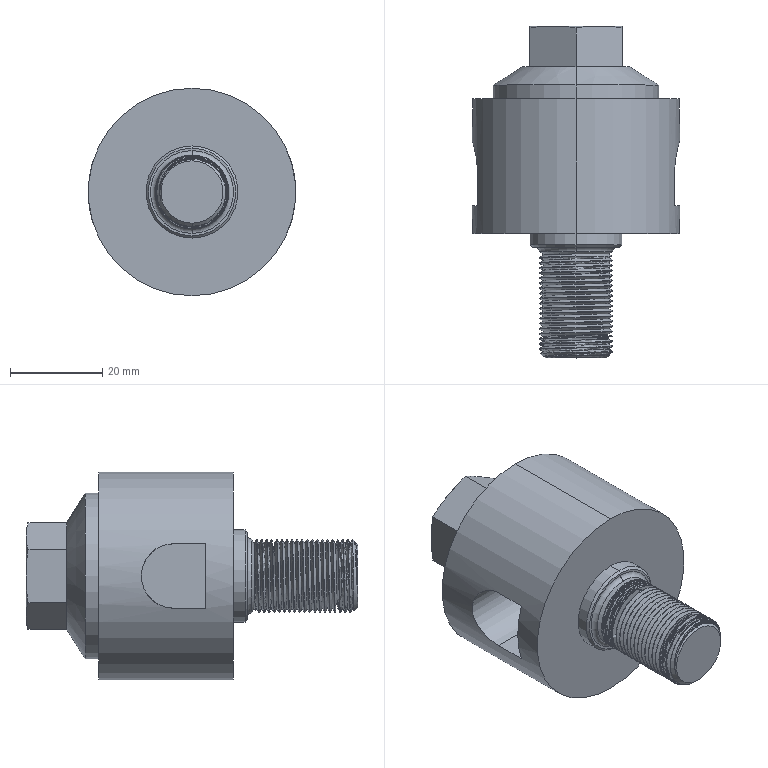Part | STEP file | Parafuso DSR-C - M16 | 1 solid | 96 faces | box 45 x 72 x 45 mm | volume 55144 mm3 | cylinder 47 | plane 27 | cone 18 | torus 2 | spline 2 | commonest cylinder face diameters 16 x39 14 x2 20 x2 36 x2 45 x2